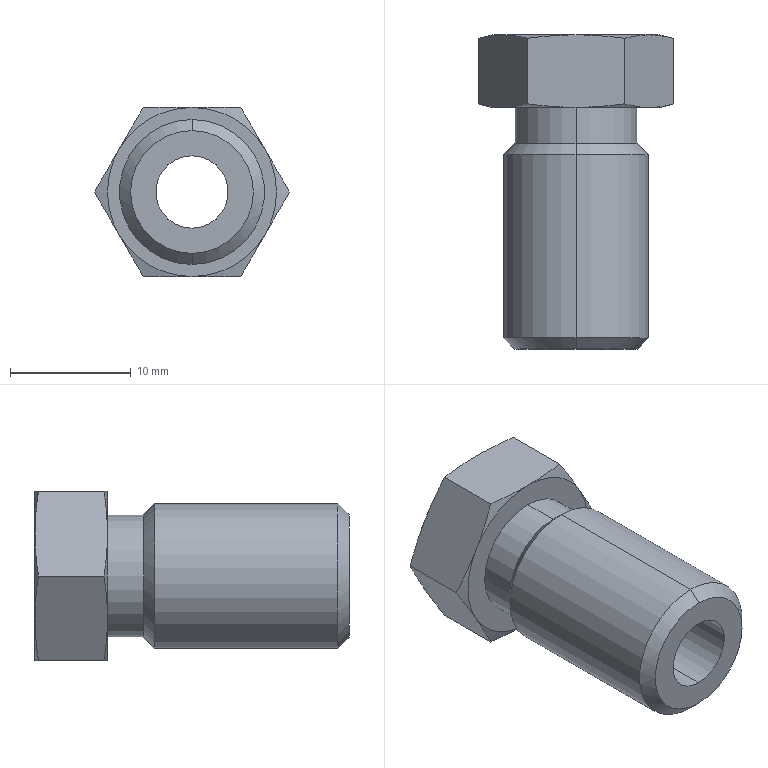Part | SolidWorks | features BaseBody 1 | 1 solid | 32 faces | box 16.166 x 26 x 14 mm | volume 2413 mm3 | cone 16 | plane 10 | cylinder 6 | commonest cylinder face diameters 6 x2 10.1 x2 12 x2
STEP:
#1=CARTESIAN_POINT('',(0.,16.08,-6.));
#2=VERTEX_POINT('',#1);
#3=CARTESIAN_POINT('',(0.,16.08,6.));
#4=VERTEX_POINT('',#3);
#5=CARTESIAN_POINT('',(0.,16.08,0.));
#6=DIRECTION('',(0.,-1.,0.));
#7=DIRECTION('',(0.,0.,-1.));
#8=AXIS2_PLACEMENT_3D('',#5,#6,#7);
#9=CIRCLE('',#8,6.);
#10=EDGE_CURVE('',#2,#4,#9,.T.);
#11=ORIENTED_EDGE('',*,*,#10,.T.);
#12=CARTESIAN_POINT('',(0.,0.92,6.));
#13=VERTEX_POINT('',#12);
#14=CARTESIAN_POINT('',(0.,8.5,6.));
#15=DIRECTION('',(0.,-1.,0.));
#16=VECTOR('',#15,1000.);
#17=LINE('',#14,#16);
#18=EDGE_CURVE('',#4,#13,#17,.T.);
#19=ORIENTED_EDGE('',*,*,#18,.T.);
#20=CARTESIAN_POINT('',(0.,0.92,-6.));
#21=VERTEX_POINT('',#20);
#22=CARTESIAN_POINT('',(0.,0.92,0.));
#23=DIRECTION('',(0.,1.,0.));
#24=DIRECTION('',(0.,0.,-1.));
#25=AXIS2_PLACEMENT_3D('',#22,#23,#24);
#26=CIRCLE('',#25,6.);
#27=EDGE_CURVE('',#13,#21,#26,.T.);
#28=ORIENTED_EDGE('',*,*,#27,.T.);
#29=CARTESIAN_POINT('',(0.,8.5,-6.));
#30=DIRECTION('',(0.,-1.,0.));
#31=VECTOR('',#30,1000.);
#32=LINE('',#29,#31);
#33=EDGE_CURVE('',#2,#21,#32,.T.);
#34=ORIENTED_EDGE('',*,*,#33,.F.);
#35=EDGE_LOOP('',(#11,#19,#28,#34));
#36=FACE_OUTER_BOUND('',#35,.T.);
#37=CARTESIAN_POINT('',(0.,8.5,0.));
#38=DIRECTION('',(0.,-1.,0.));
#39=DIRECTION('',(0.,0.,-1.));
#40=AXIS2_PLACEMENT_3D('',#37,#38,#39);
#41=CYLINDRICAL_SURFACE('',#40,6.);
#42=ADVANCED_FACE('',(#36),#41,.T.);
#43=CARTESIAN_POINT('',(0.,17.,-5.08));
#44=VERTEX_POINT('',#43);
#45=CARTESIAN_POINT('',(0.,17.,5.08));
#46=VERTEX_POINT('',#45);
#47=CARTESIAN_POINT('',(0.,17.,0.));
#48=DIRECTION('',(0.,-1.,0.));
#49=DIRECTION('',(0.,0.,-1.));
#50=AXIS2_PLACEMENT_3D('',#47,#48,#49);
#51=CIRCLE('',#50,5.08);
#52=EDGE_CURVE('',#44,#46,#51,.T.);
#53=ORIENTED_EDGE('',*,*,#52,.T.);
#54=CARTESIAN_POINT('',(0.,16.08,6.));
#55=DIRECTION('',(0.,-0.7071,0.7071));
#56=VECTOR('',#55,1000.);
#57=LINE('',#54,#56);
#58=EDGE_CURVE('',#46,#4,#57,.T.);
#59=ORIENTED_EDGE('',*,*,#58,.T.);
#60=ORIENTED_EDGE('',*,*,#10,.F.);
#61=CARTESIAN_POINT('',(0.,16.08,-6.));
#62=DIRECTION('',(0.,-0.7071,-0.7071));
#63=VECTOR('',#62,1000.);
#64=LINE('',#61,#63);
#65=EDGE_CURVE('',#44,#2,#64,.T.);
#66=ORIENTED_EDGE('',*,*,#65,.F.);
#67=EDGE_LOOP('',(#53,#59,#60,#66));
#68=FACE_OUTER_BOUND('',#67,.T.);
#69=CARTESIAN_POINT('',(0.,16.08,0.));
#70=DIRECTION('',(0.,-1.,0.));
#71=DIRECTION('',(0.,0.,-1.));
#72=AXIS2_PLACEMENT_3D('',#69,#70,#71);
#73=CONICAL_SURFACE('',#72,6.,0.7854);
#74=ADVANCED_FACE('',(#68),#73,.T.);
#75=CARTESIAN_POINT('',(0.,0.,5.08));
#76=VERTEX_POINT('',#75);
#77=CARTESIAN_POINT('',(0.,0.,-5.08));
#78=VERTEX_POINT('',#77);
#79=CARTESIAN_POINT('',(0.,0.,0.));
#80=DIRECTION('',(0.,1.,0.));
#81=DIRECTION('',(0.,0.,1.));
#82=AXIS2_PLACEMENT_3D('',#79,#80,#81);
#83=CIRCLE('',#82,5.08);
#84=EDGE_CURVE('',#76,#78,#83,.T.);
#85=ORIENTED_EDGE('',*,*,#84,.T.);
#86=CARTESIAN_POINT('',(0.,0.92,-6.));
#87=DIRECTION('',(0.,0.7071,-0.7071));
#88=VECTOR('',#87,1000.);
#89=LINE('',#86,#88);
#90=EDGE_CURVE('',#78,#21,#89,.T.);
#91=ORIENTED_EDGE('',*,*,#90,.T.);
#92=ORIENTED_EDGE('',*,*,#27,.F.);
#93=CARTESIAN_POINT('',(0.,0.92,6.));
#94=DIRECTION('',(0.,0.7071,0.7071));
#95=VECTOR('',#94,1000.);
#96=LINE('',#93,#95);
#97=EDGE_CURVE('',#76,#13,#96,.T.);
#98=ORIENTED_EDGE('',*,*,#97,.F.);
#99=EDGE_LOOP('',(#85,#91,#92,#98));
#100=FACE_OUTER_BOUND('',#99,.T.);
#101=CARTESIAN_POINT('',(0.,0.92,0.));
#102=DIRECTION('',(0.,1.,0.));
#103=DIRECTION('',(0.,0.,1.));
#104=AXIS2_PLACEMENT_3D('',#101,#102,#103);
#105=CONICAL_SURFACE('',#104,6.,0.7854);
#106=ADVANCED_FACE('',(#100),#105,.T.);
#107=CARTESIAN_POINT('',(0.,20.,-5.05));
#108=VERTEX_POINT('',#107);
#109=CARTESIAN_POINT('',(0.,20.,5.05));
#110=VERTEX_POINT('',#109);
#111=CARTESIAN_POINT('',(0.,20.,0.));
#112=DIRECTION('',(0.,-1.,0.));
#113=DIRECTION('',(0.,0.,-1.));
#114=AXIS2_PLACEMENT_3D('',#111,#112,#113);
#115=CIRCLE('',#114,5.05);
#116=EDGE_CURVE('',#108,#110,#115,.T.);
#117=ORIENTED_EDGE('',*,*,#116,.T.);
#118=CARTESIAN_POINT('',(0.,17.,5.05));
#119=VERTEX_POINT('',#118);
#120=CARTESIAN_POINT('',(0.,18.5,5.05));
#121=DIRECTION('',(0.,-1.,0.));
#122=VECTOR('',#121,1000.);
#123=LINE('',#120,#122);
#124=EDGE_CURVE('',#110,#119,#123,.T.);
#125=ORIENTED_EDGE('',*,*,#124,.T.);
#126=CARTESIAN_POINT('',(0.,17.,-5.05));
#127=VERTEX_POINT('',#126);
#128=CARTESIAN_POINT('',(0.,17.,0.));
#129=DIRECTION('',(0.,-1.,0.));
#130=DIRECTION('',(0.,0.,-1.));
#131=AXIS2_PLACEMENT_3D('',#128,#129,#130);
#132=CIRCLE('',#131,5.05);
#133=EDGE_CURVE('',#127,#119,#132,.T.);
#134=ORIENTED_EDGE('',*,*,#133,.F.);
#135=CARTESIAN_POINT('',(0.,18.5,-5.05));
#136=DIRECTION('',(0.,-1.,0.));
#137=VECTOR('',#136,1000.);
#138=LINE('',#135,#137);
#139=EDGE_CURVE('',#108,#127,#138,.T.);
#140=ORIENTED_EDGE('',*,*,#139,.F.);
#141=EDGE_LOOP('',(#117,#125,#134,#140));
#142=FACE_OUTER_BOUND('',#141,.T.);
#143=CARTESIAN_POINT('',(0.,18.5,0.));
#144=DIRECTION('',(0.,-1.,0.));
#145=DIRECTION('',(0.,0.,-1.));
#146=AXIS2_PLACEMENT_3D('',#143,#144,#145);
#147=CYLINDRICAL_SURFACE('',#146,5.05);
#148=ADVANCED_FACE('',(#142),#147,.T.);
#149=CARTESIAN_POINT('',(0.,26.,3.));
#150=VERTEX_POINT('',#149);
#151=CARTESIAN_POINT('',(0.,26.,-3.));
#152=VERTEX_POINT('',#151);
#153=CARTESIAN_POINT('',(0.,26.,0.));
#154=DIRECTION('',(0.,-1.,0.));
#155=DIRECTION('',(0.,0.,-1.));
#156=AXIS2_PLACEMENT_3D('',#153,#154,#155);
#157=CIRCLE('',#156,3.);
#158=EDGE_CURVE('',#150,#152,#157,.T.);
#159=ORIENTED_EDGE('',*,*,#158,.F.);
#160=CARTESIAN_POINT('',(0.,0.,3.));
#161=VERTEX_POINT('',#160);
#162=CARTESIAN_POINT('',(0.,13.,3.));
#163=DIRECTION('',(0.,-1.,0.));
#164=VECTOR('',#163,1000.);
#165=LINE('',#162,#164);
#166=EDGE_CURVE('',#150,#161,#165,.T.);
#167=ORIENTED_EDGE('',*,*,#166,.T.);
#168=CARTESIAN_POINT('',(0.,0.,-3.));
#169=VERTEX_POINT('',#168);
#170=CARTESIAN_POINT('',(0.,0.,0.));
#171=DIRECTION('',(0.,1.,0.));
#172=DIRECTION('',(0.,0.,-1.));
#173=AXIS2_PLACEMENT_3D('',#170,#171,#172);
#174=CIRCLE('',#173,3.);
#175=EDGE_CURVE('',#169,#161,#174,.T.);
#176=ORIENTED_EDGE('',*,*,#175,.F.);
#177=CARTESIAN_POINT('',(0.,13.,-3.));
#178=DIRECTION('',(0.,-1.,0.));
#179=VECTOR('',#178,1000.);
#180=LINE('',#177,#179);
#181=EDGE_CURVE('',#152,#169,#180,.T.);
#182=ORIENTED_EDGE('',*,*,#181,.F.);
#183=EDGE_LOOP('',(#159,#167,#176,#182));
#184=FACE_OUTER_BOUND('',#183,.T.);
#185=CARTESIAN_POINT('',(0.,13.,0.));
#186=DIRECTION('',(0.,-1.,0.));
#187=DIRECTION('',(0.,0.,-1.));
#188=AXIS2_PLACEMENT_3D('',#185,#186,#187);
#189=CYLINDRICAL_SURFACE('',#188,3.);
#190=ADVANCED_FACE('',(#184),#189,.F.);
#191=ORIENTED_EDGE('',*,*,#18,.F.);
#192=CARTESIAN_POINT('',(0.,16.08,0.));
#193=DIRECTION('',(0.,-1.,0.));
#194=DIRECTION('',(0.,0.,-1.));
#195=AXIS2_PLACEMENT_3D('',#192,#193,#194);
#196=CIRCLE('',#195,6.);
#197=EDGE_CURVE('',#4,#2,#196,.T.);
#198=ORIENTED_EDGE('',*,*,#197,.T.);
#199=ORIENTED_EDGE('',*,*,#33,.T.);
#200=CARTESIAN_POINT('',(0.,0.92,0.));
#201=DIRECTION('',(0.,1.,0.));
#202=DIRECTION('',(0.,0.,-1.));
#203=AXIS2_PLACEMENT_3D('',#200,#201,#202);
#204=CIRCLE('',#203,6.);
#205=EDGE_CURVE('',#21,#13,#204,.T.);
#206=ORIENTED_EDGE('',*,*,#205,.T.);
#207=EDGE_LOOP('',(#191,#198,#199,#206));
#208=FACE_OUTER_BOUND('',#207,.T.);
#209=CARTESIAN_POINT('',(0.,8.5,0.));
#210=DIRECTION('',(0.,-1.,0.));
#211=DIRECTION('',(0.,0.,-1.));
#212=AXIS2_PLACEMENT_3D('',#209,#210,#211);
#213=CYLINDRICAL_SURFACE('',#212,6.);
#214=ADVANCED_FACE('',(#208),#213,.T.);
#215=ORIENTED_EDGE('',*,*,#58,.F.);
#216=CARTESIAN_POINT('',(0.,17.,0.));
#217=DIRECTION('',(0.,-1.,0.));
#218=DIRECTION('',(0.,0.,-1.));
#219=AXIS2_PLACEMENT_3D('',#216,#217,#218);
#220=CIRCLE('',#219,5.08);
#221=EDGE_CURVE('',#46,#44,#220,.T.);
#222=ORIENTED_EDGE('',*,*,#221,.T.);
#223=ORIENTED_EDGE('',*,*,#65,.T.);
#224=ORIENTED_EDGE('',*,*,#197,.F.);
#225=EDGE_LOOP('',(#215,#222,#223,#224));
#226=FACE_OUTER_BOUND('',#225,.T.);
#227=CARTESIAN_POINT('',(0.,16.08,0.));
#228=DIRECTION('',(0.,-1.,0.));
#229=DIRECTION('',(0.,0.,-1.));
#230=AXIS2_PLACEMENT_3D('',#227,#228,#229);
#231=CONICAL_SURFACE('',#230,6.,0.7854);
#232=ADVANCED_FACE('',(#226),#231,.T.);
#233=ORIENTED_EDGE('',*,*,#90,.F.);
#234=CARTESIAN_POINT('',(0.,0.,0.));
#235=DIRECTION('',(0.,1.,0.));
#236=DIRECTION('',(0.,0.,1.));
#237=AXIS2_PLACEMENT_3D('',#234,#235,#236);
#238=CIRCLE('',#237,5.08);
#239=EDGE_CURVE('',#78,#76,#238,.T.);
#240=ORIENTED_EDGE('',*,*,#239,.T.);
#241=ORIENTED_EDGE('',*,*,#97,.T.);
#242=ORIENTED_EDGE('',*,*,#205,.F.);
#243=EDGE_LOOP('',(#233,#240,#241,#242));
#244=FACE_OUTER_BOUND('',#243,.T.);
#245=CARTESIAN_POINT('',(0.,0.92,0.));
#246=DIRECTION('',(0.,1.,0.));
#247=DIRECTION('',(0.,0.,1.));
#248=AXIS2_PLACEMENT_3D('',#245,#246,#247);
#249=CONICAL_SURFACE('',#248,6.,0.7854);
#250=ADVANCED_FACE('',(#244),#249,.T.);
#251=ORIENTED_EDGE('',*,*,#52,.F.);
#252=ORIENTED_EDGE('',*,*,#221,.F.);
#253=EDGE_LOOP('',(#251,#252));
#254=FACE_OUTER_BOUND('',#253,.T.);
#255=ORIENTED_EDGE('',*,*,#133,.T.);
#256=CARTESIAN_POINT('',(0.,17.,0.));
#257=DIRECTION('',(0.,-1.,0.));
#258=DIRECTION('',(0.,0.,-1.));
#259=AXIS2_PLACEMENT_3D('',#256,#257,#258);
#260=CIRCLE('',#259,5.05);
#261=EDGE_CURVE('',#119,#127,#260,.T.);
#262=ORIENTED_EDGE('',*,*,#261,.T.);
#263=EDGE_LOOP('',(#255,#262));
#264=FACE_BOUND('',#263,.T.);
#265=CARTESIAN_POINT('',(5.065,17.,0.));
#266=DIRECTION('',(0.,1.,0.));
#267=DIRECTION('',(0.,0.,1.));
#268=AXIS2_PLACEMENT_3D('',#265,#266,#267);
#269=PLANE('',#268);
#270=ADVANCED_FACE('',(#254,#264),#269,.T.);
#271=ORIENTED_EDGE('',*,*,#84,.F.);
#272=ORIENTED_EDGE('',*,*,#239,.F.);
#273=EDGE_LOOP('',(#271,#272));
#274=FACE_OUTER_BOUND('',#273,.T.);
#275=ORIENTED_EDGE('',*,*,#175,.T.);
#276=CARTESIAN_POINT('',(0.,0.,0.));
#277=DIRECTION('',(0.,1.,0.));
#278=DIRECTION('',(0.,0.,-1.));
#279=AXIS2_PLACEMENT_3D('',#276,#277,#278);
#280=CIRCLE('',#279,3.);
#281=EDGE_CURVE('',#161,#169,#280,.T.);
#282=ORIENTED_EDGE('',*,*,#281,.T.);
#283=EDGE_LOOP('',(#275,#282));
#284=FACE_BOUND('',#283,.T.);
#285=CARTESIAN_POINT('',(2.54,0.,0.));
#286=DIRECTION('',(0.,-1.,0.));
#287=DIRECTION('',(0.,0.,-1.));
#288=AXIS2_PLACEMENT_3D('',#285,#286,#287);
#289=PLANE('',#288);
#290=ADVANCED_FACE('',(#274,#284),#289,.T.);
#291=ORIENTED_EDGE('',*,*,#124,.F.);
#292=CARTESIAN_POINT('',(0.,20.,0.));
#293=DIRECTION('',(0.,-1.,0.));
#294=DIRECTION('',(0.,0.,-1.));
#295=AXIS2_PLACEMENT_3D('',#292,#293,#294);
#296=CIRCLE('',#295,5.05);
#297=EDGE_CURVE('',#110,#108,#296,.T.);
#298=ORIENTED_EDGE('',*,*,#297,.T.);
#299=ORIENTED_EDGE('',*,*,#139,.T.);
#300=ORIENTED_EDGE('',*,*,#261,.F.);
#301=EDGE_LOOP('',(#291,#298,#299,#300));
#302=FACE_OUTER_BOUND('',#301,.T.);
#303=CARTESIAN_POINT('',(0.,18.5,0.));
#304=DIRECTION('',(0.,-1.,0.));
#305=DIRECTION('',(0.,0.,-1.));
#306=AXIS2_PLACEMENT_3D('',#303,#304,#305);
#307=CYLINDRICAL_SURFACE('',#306,5.05);
#308=ADVANCED_FACE('',(#302),#307,.T.);
#309=ORIENTED_EDGE('',*,*,#166,.F.);
#310=CARTESIAN_POINT('',(0.,26.,0.));
#311=DIRECTION('',(0.,-1.,0.));
#312=DIRECTION('',(0.,0.,-1.));
#313=AXIS2_PLACEMENT_3D('',#310,#311,#312);
#314=CIRCLE('',#313,3.);
#315=EDGE_CURVE('',#152,#150,#314,.T.);
#316=ORIENTED_EDGE('',*,*,#315,.F.);
#317=ORIENTED_EDGE('',*,*,#181,.T.);
#318=ORIENTED_EDGE('',*,*,#281,.F.);
#319=EDGE_LOOP('',(#309,#316,#317,#318));
#320=FACE_OUTER_BOUND('',#319,.T.);
#321=CARTESIAN_POINT('',(0.,13.,0.));
#322=DIRECTION('',(0.,-1.,0.));
#323=DIRECTION('',(0.,0.,-1.));
#324=AXIS2_PLACEMENT_3D('',#321,#322,#323);
#325=CYLINDRICAL_SURFACE('',#324,3.);
#326=ADVANCED_FACE('',(#320),#325,.F.);
#327=ORIENTED_EDGE('',*,*,#116,.F.);
#328=ORIENTED_EDGE('',*,*,#297,.F.);
#329=EDGE_LOOP('',(#327,#328));
#330=FACE_BOUND('',#329,.T.);
#331=CARTESIAN_POINT('',(0.,20.,-7.));
#332=VERTEX_POINT('',#331);
#333=CARTESIAN_POINT('',(6.062,20.,-3.5));
#334=VERTEX_POINT('',#333);
#335=CARTESIAN_POINT('',(0.,20.,0.));
#336=DIRECTION('',(0.,-1.,0.));
#337=DIRECTION('',(0.,0.,1.));
#338=AXIS2_PLACEMENT_3D('',#335,#336,#337);
#339=CIRCLE('',#338,7.);
#340=EDGE_CURVE('',#332,#334,#339,.T.);
#341=ORIENTED_EDGE('',*,*,#340,.T.);
#342=CARTESIAN_POINT('',(6.062,20.,3.5));
#343=VERTEX_POINT('',#342);
#344=CARTESIAN_POINT('',(0.,20.,0.));
#345=DIRECTION('',(0.,-1.,0.));
#346=DIRECTION('',(0.,0.,1.));
#347=AXIS2_PLACEMENT_3D('',#344,#345,#346);
#348=CIRCLE('',#347,7.);
#349=EDGE_CURVE('',#334,#343,#348,.T.);
#350=ORIENTED_EDGE('',*,*,#349,.T.);
#351=CARTESIAN_POINT('',(0.,20.,7.));
#352=VERTEX_POINT('',#351);
#353=CARTESIAN_POINT('',(0.,20.,0.));
#354=DIRECTION('',(0.,-1.,0.));
#355=DIRECTION('',(0.,0.,1.));
#356=AXIS2_PLACEMENT_3D('',#353,#354,#355);
#357=CIRCLE('',#356,7.);
#358=EDGE_CURVE('',#343,#352,#357,.T.);
#359=ORIENTED_EDGE('',*,*,#358,.T.);
#360=CARTESIAN_POINT('',(-6.062,20.,3.5));
#361=VERTEX_POINT('',#360);
#362=CARTESIAN_POINT('',(0.,20.,0.));
#363=DIRECTION('',(0.,-1.,0.));
#364=DIRECTION('',(0.,0.,1.));
#365=AXIS2_PLACEMENT_3D('',#362,#363,#364);
#366=CIRCLE('',#365,7.);
#367=EDGE_CURVE('',#352,#361,#366,.T.);
#368=ORIENTED_EDGE('',*,*,#367,.T.);
#369=CARTESIAN_POINT('',(-6.062,20.,-3.5));
#370=VERTEX_POINT('',#369);
#371=CARTESIAN_POINT('',(0.,20.,0.));
#372=DIRECTION('',(0.,-1.,0.));
#373=DIRECTION('',(0.,0.,1.));
#374=AXIS2_PLACEMENT_3D('',#371,#372,#373);
#375=CIRCLE('',#374,7.);
#376=EDGE_CURVE('',#361,#370,#375,.T.);
#377=ORIENTED_EDGE('',*,*,#376,.T.);
#378=CARTESIAN_POINT('',(0.,20.,0.));
#379=DIRECTION('',(0.,-1.,0.));
#380=DIRECTION('',(0.,0.,1.));
#381=AXIS2_PLACEMENT_3D('',#378,#379,#380);
#382=CIRCLE('',#381,7.);
#383=EDGE_CURVE('',#370,#332,#382,.T.);
#384=ORIENTED_EDGE('',*,*,#383,.T.);
#385=EDGE_LOOP('',(#341,#350,#359,#368,#377,#384));
#386=FACE_OUTER_BOUND('',#385,.T.);
#387=CARTESIAN_POINT('',(6.025,20.,0.));
#388=DIRECTION('',(0.,-1.,0.));
#389=DIRECTION('',(0.,0.,-1.));
#390=AXIS2_PLACEMENT_3D('',#387,#388,#389);
#391=PLANE('',#390);
#392=ADVANCED_FACE('',(#330,#386),#391,.T.);
#393=CARTESIAN_POINT('',(-6.062,26.,3.5));
#394=VERTEX_POINT('',#393);
#395=CARTESIAN_POINT('',(0.,26.,7.));
#396=VERTEX_POINT('',#395);
#397=CARTESIAN_POINT('',(0.,26.,0.));
#398=DIRECTION('',(0.,1.,0.));
#399=DIRECTION('',(0.,0.,-1.));
#400=AXIS2_PLACEMENT_3D('',#397,#398,#399);
#401=CIRCLE('',#400,7.);
#402=EDGE_CURVE('',#394,#396,#401,.T.);
#403=ORIENTED_EDGE('',*,*,#402,.T.);
#404=CARTESIAN_POINT('',(6.062,26.,3.5));
#405=VERTEX_POINT('',#404);
#406=CARTESIAN_POINT('',(0.,26.,0.));
#407=DIRECTION('',(0.,1.,0.));
#408=DIRECTION('',(0.,0.,-1.));
#409=AXIS2_PLACEMENT_3D('',#406,#407,#408);
#410=CIRCLE('',#409,7.);
#411=EDGE_CURVE('',#396,#405,#410,.T.);
#412=ORIENTED_EDGE('',*,*,#411,.T.);
#413=CARTESIAN_POINT('',(6.062,26.,-3.5));
#414=VERTEX_POINT('',#413);
#415=CARTESIAN_POINT('',(0.,26.,0.));
#416=DIRECTION('',(0.,1.,0.));
#417=DIRECTION('',(0.,0.,-1.));
#418=AXIS2_PLACEMENT_3D('',#415,#416,#417);
#419=CIRCLE('',#418,7.);
#420=EDGE_CURVE('',#405,#414,#419,.T.);
#421=ORIENTED_EDGE('',*,*,#420,.T.);
#422=CARTESIAN_POINT('',(0.,26.,-7.));
#423=VERTEX_POINT('',#422);
#424=CARTESIAN_POINT('',(0.,26.,0.));
#425=DIRECTION('',(0.,1.,0.));
#426=DIRECTION('',(0.,0.,-1.));
#427=AXIS2_PLACEMENT_3D('',#424,#425,#426);
#428=CIRCLE('',#427,7.);
#429=EDGE_CURVE('',#414,#423,#428,.T.);
#430=ORIENTED_EDGE('',*,*,#429,.T.);
#431=CARTESIAN_POINT('',(-6.062,26.,-3.5));
#432=VERTEX_POINT('',#431);
#433=CARTESIAN_POINT('',(0.,26.,0.));
#434=DIRECTION('',(0.,1.,0.));
#435=DIRECTION('',(0.,0.,-1.));
#436=AXIS2_PLACEMENT_3D('',#433,#434,#435);
#437=CIRCLE('',#436,7.);
#438=EDGE_CURVE('',#423,#432,#437,.T.);
#439=ORIENTED_EDGE('',*,*,#438,.T.);
#440=CARTESIAN_POINT('',(0.,26.,0.));
#441=DIRECTION('',(0.,1.,0.));
#442=DIRECTION('',(0.,0.,-1.));
#443=AXIS2_PLACEMENT_3D('',#440,#441,#442);
#444=CIRCLE('',#443,7.);
#445=EDGE_CURVE('',#432,#394,#444,.T.);
#446=ORIENTED_EDGE('',*,*,#445,.T.);
#447=EDGE_LOOP('',(#403,#412,#421,#430,#439,#446));
#448=FACE_OUTER_BOUND('',#447,.T.);
#449=ORIENTED_EDGE('',*,*,#315,.T.);
#450=ORIENTED_EDGE('',*,*,#158,.T.);
#451=EDGE_LOOP('',(#449,#450));
#452=FACE_BOUND('',#451,.T.);
#453=CARTESIAN_POINT('',(3.5,26.,0.));
#454=DIRECTION('',(0.,1.,0.));
#455=DIRECTION('',(0.,0.,1.));
#456=AXIS2_PLACEMENT_3D('',#453,#454,#455);
#457=PLANE('',#456);
#458=ADVANCED_FACE('',(#448,#452),#457,.T.);
#459=ORIENTED_EDGE('',*,*,#349,.F.);
#460=CARTESIAN_POINT('',(8.083,20.29,0.));
#461=VERTEX_POINT('',#460);
#462=CARTESIAN_POINT('',(6.062,20.,-3.5));
#463=CARTESIAN_POINT('',(6.739,20.,-2.327));
#464=CARTESIAN_POINT('',(7.412,20.11,-1.162));
#465=CARTESIAN_POINT('',(8.083,20.29,0.));
#466=B_SPLINE_CURVE_WITH_KNOTS('',3,(#462,#463,#464,#465),.UNSPECIFIED.,.F.,.F.,(4,4),(0.,0.004052),.UNSPECIFIED.);
#467=EDGE_CURVE('',#334,#461,#466,.T.);
#468=ORIENTED_EDGE('',*,*,#467,.T.);
#469=CARTESIAN_POINT('',(8.083,20.29,0.));
#470=CARTESIAN_POINT('',(7.412,20.11,1.162));
#471=CARTESIAN_POINT('',(6.739,20.,2.327));
#472=CARTESIAN_POINT('',(6.062,20.,3.5));
#473=B_SPLINE_CURVE_WITH_KNOTS('',3,(#469,#470,#471,#472),.UNSPECIFIED.,.F.,.F.,(4,4),(0.,0.004052),.UNSPECIFIED.);
#474=EDGE_CURVE('',#461,#343,#473,.T.);
#475=ORIENTED_EDGE('',*,*,#474,.T.);
#476=EDGE_LOOP('',(#459,#468,#475));
#477=FACE_OUTER_BOUND('',#476,.T.);
#478=CARTESIAN_POINT('',(0.,20.292,0.));
#479=DIRECTION('',(0.,1.,0.));
#480=DIRECTION('',(0.,0.,1.));
#481=AXIS2_PLACEMENT_3D('',#478,#479,#480);
#482=CONICAL_SURFACE('',#481,8.089,1.309);
#483=ADVANCED_FACE('',(#477),#482,.T.);
#484=ORIENTED_EDGE('',*,*,#340,.F.);
#485=CARTESIAN_POINT('',(4.041,20.29,-7.));
#486=VERTEX_POINT('',#485);
#487=CARTESIAN_POINT('',(0.,20.,-7.));
#488=CARTESIAN_POINT('',(1.354,20.,-7.));
#489=CARTESIAN_POINT('',(2.7,20.11,-7.));
#490=CARTESIAN_POINT('',(4.041,20.29,-7.));
#491=B_SPLINE_CURVE_WITH_KNOTS('',3,(#487,#488,#489,#490),.UNSPECIFIED.,.F.,.F.,(4,4),(0.,0.004052),.UNSPECIFIED.);
#492=EDGE_CURVE('',#332,#486,#491,.T.);
#493=ORIENTED_EDGE('',*,*,#492,.T.);
#494=CARTESIAN_POINT('',(4.041,20.29,-7.));
#495=CARTESIAN_POINT('',(4.712,20.11,-5.838));
#496=CARTESIAN_POINT('',(5.385,20.,-4.673));
#497=CARTESIAN_POINT('',(6.062,20.,-3.5));
#498=B_SPLINE_CURVE_WITH_KNOTS('',3,(#494,#495,#496,#497),.UNSPECIFIED.,.F.,.F.,(4,4),(0.,0.004052),.UNSPECIFIED.);
#499=EDGE_CURVE('',#486,#334,#498,.T.);
#500=ORIENTED_EDGE('',*,*,#499,.T.);
#501=EDGE_LOOP('',(#484,#493,#500));
#502=FACE_OUTER_BOUND('',#501,.T.);
#503=CARTESIAN_POINT('',(0.,20.292,0.));
#504=DIRECTION('',(0.,1.,0.));
#505=DIRECTION('',(0.,0.,1.));
#506=AXIS2_PLACEMENT_3D('',#503,#504,#505);
#507=CONICAL_SURFACE('',#506,8.089,1.309);
#508=ADVANCED_FACE('',(#502),#507,.T.);
#509=CARTESIAN_POINT('',(-4.041,20.29,-7.));
#510=VERTEX_POINT('',#509);
#511=CARTESIAN_POINT('',(-4.041,20.29,-7.));
#512=CARTESIAN_POINT('',(-2.7,20.11,-7.));
#513=CARTESIAN_POINT('',(-1.354,20.,-7.));
#514=CARTESIAN_POINT('',(0.,20.,-7.));
#515=B_SPLINE_CURVE_WITH_KNOTS('',3,(#511,#512,#513,#514),.UNSPECIFIED.,.F.,.F.,(4,4),(0.,0.004052),.UNSPECIFIED.);
#516=EDGE_CURVE('',#510,#332,#515,.T.);
#517=ORIENTED_EDGE('',*,*,#516,.T.);
#518=ORIENTED_EDGE('',*,*,#383,.F.);
#519=CARTESIAN_POINT('',(-6.062,20.,-3.5));
#520=CARTESIAN_POINT('',(-5.385,20.,-4.673));
#521=CARTESIAN_POINT('',(-4.712,20.11,-5.838));
#522=CARTESIAN_POINT('',(-4.041,20.29,-7.));
#523=B_SPLINE_CURVE_WITH_KNOTS('',3,(#519,#520,#521,#522),.UNSPECIFIED.,.F.,.F.,(4,4),(0.,0.004052),.UNSPECIFIED.);
#524=EDGE_CURVE('',#370,#510,#523,.T.);
#525=ORIENTED_EDGE('',*,*,#524,.T.);
#526=EDGE_LOOP('',(#517,#518,#525));
#527=FACE_OUTER_BOUND('',#526,.T.);
#528=CARTESIAN_POINT('',(0.,20.292,0.));
#529=DIRECTION('',(0.,1.,0.));
#530=DIRECTION('',(0.,0.,1.));
#531=AXIS2_PLACEMENT_3D('',#528,#529,#530);
#532=CONICAL_SURFACE('',#531,8.089,1.309);
#533=ADVANCED_FACE('',(#527),#532,.T.);
#534=CARTESIAN_POINT('',(-8.083,20.29,0.));
#535=VERTEX_POINT('',#534);
#536=CARTESIAN_POINT('',(-8.083,20.29,0.));
#537=CARTESIAN_POINT('',(-7.412,20.11,-1.162));
#538=CARTESIAN_POINT('',(-6.739,20.,-2.327));
#539=CARTESIAN_POINT('',(-6.062,20.,-3.5));
#540=B_SPLINE_CURVE_WITH_KNOTS('',3,(#536,#537,#538,#539),.UNSPECIFIED.,.F.,.F.,(4,4),(0.,0.004052),.UNSPECIFIED.);
#541=EDGE_CURVE('',#535,#370,#540,.T.);
#542=ORIENTED_EDGE('',*,*,#541,.T.);
#543=ORIENTED_EDGE('',*,*,#376,.F.);
#544=CARTESIAN_POINT('',(-6.062,20.,3.5));
#545=CARTESIAN_POINT('',(-6.739,20.,2.327));
#546=CARTESIAN_POINT('',(-7.412,20.11,1.162));
#547=CARTESIAN_POINT('',(-8.083,20.29,0.));
#548=B_SPLINE_CURVE_WITH_KNOTS('',3,(#544,#545,#546,#547),.UNSPECIFIED.,.F.,.F.,(4,4),(0.,0.004052),.UNSPECIFIED.);
#549=EDGE_CURVE('',#361,#535,#548,.T.);
#550=ORIENTED_EDGE('',*,*,#549,.T.);
#551=EDGE_LOOP('',(#542,#543,#550));
#552=FACE_OUTER_BOUND('',#551,.T.);
#553=CARTESIAN_POINT('',(0.,20.292,0.));
#554=DIRECTION('',(0.,1.,0.));
#555=DIRECTION('',(0.,0.,1.));
#556=AXIS2_PLACEMENT_3D('',#553,#554,#555);
#557=CONICAL_SURFACE('',#556,8.089,1.309);
#558=ADVANCED_FACE('',(#552),#557,.T.);
#559=CARTESIAN_POINT('',(-4.041,20.29,7.));
#560=VERTEX_POINT('',#559);
#561=CARTESIAN_POINT('',(-4.041,20.29,7.));
#562=CARTESIAN_POINT('',(-4.712,20.11,5.838));
#563=CARTESIAN_POINT('',(-5.385,20.,4.673));
#564=CARTESIAN_POINT('',(-6.062,20.,3.5));
#565=B_SPLINE_CURVE_WITH_KNOTS('',3,(#561,#562,#563,#564),.UNSPECIFIED.,.F.,.F.,(4,4),(0.,0.004052),.UNSPECIFIED.);
#566=EDGE_CURVE('',#560,#361,#565,.T.);
#567=ORIENTED_EDGE('',*,*,#566,.T.);
#568=ORIENTED_EDGE('',*,*,#367,.F.);
#569=CARTESIAN_POINT('',(0.,20.,7.));
#570=CARTESIAN_POINT('',(-1.354,20.,7.));
#571=CARTESIAN_POINT('',(-2.7,20.11,7.));
#572=CARTESIAN_POINT('',(-4.041,20.29,7.));
#573=B_SPLINE_CURVE_WITH_KNOTS('',3,(#569,#570,#571,#572),.UNSPECIFIED.,.F.,.F.,(4,4),(0.,0.004052),.UNSPECIFIED.);
#574=EDGE_CURVE('',#352,#560,#573,.T.);
#575=ORIENTED_EDGE('',*,*,#574,.T.);
#576=EDGE_LOOP('',(#567,#568,#575));
#577=FACE_OUTER_BOUND('',#576,.T.);
#578=CARTESIAN_POINT('',(0.,20.292,0.));
#579=DIRECTION('',(0.,1.,0.));
#580=DIRECTION('',(0.,0.,1.));
#581=AXIS2_PLACEMENT_3D('',#578,#579,#580);
#582=CONICAL_SURFACE('',#581,8.089,1.309);
#583=ADVANCED_FACE('',(#577),#582,.T.);
#584=ORIENTED_EDGE('',*,*,#358,.F.);
#585=CARTESIAN_POINT('',(4.041,20.29,7.));
#586=VERTEX_POINT('',#585);
#587=CARTESIAN_POINT('',(6.062,20.,3.5));
#588=CARTESIAN_POINT('',(5.385,20.,4.673));
#589=CARTESIAN_POINT('',(4.712,20.11,5.838));
#590=CARTESIAN_POINT('',(4.041,20.29,7.));
#591=B_SPLINE_CURVE_WITH_KNOTS('',3,(#587,#588,#589,#590),.UNSPECIFIED.,.F.,.F.,(4,4),(0.,0.004052),.UNSPECIFIED.);
#592=EDGE_CURVE('',#343,#586,#591,.T.);
#593=ORIENTED_EDGE('',*,*,#592,.T.);
#594=CARTESIAN_POINT('',(4.041,20.29,7.));
#595=CARTESIAN_POINT('',(2.7,20.11,7.));
#596=CARTESIAN_POINT('',(1.354,20.,7.));
#597=CARTESIAN_POINT('',(0.,20.,7.));
#598=B_SPLINE_CURVE_WITH_KNOTS('',3,(#594,#595,#596,#597),.UNSPECIFIED.,.F.,.F.,(4,4),(0.,0.004052),.UNSPECIFIED.);
#599=EDGE_CURVE('',#586,#352,#598,.T.);
#600=ORIENTED_EDGE('',*,*,#599,.T.);
#601=EDGE_LOOP('',(#584,#593,#600));
#602=FACE_OUTER_BOUND('',#601,.T.);
#603=CARTESIAN_POINT('',(0.,20.292,0.));
#604=DIRECTION('',(0.,1.,0.));
#605=DIRECTION('',(0.,0.,1.));
#606=AXIS2_PLACEMENT_3D('',#603,#604,#605);
#607=CONICAL_SURFACE('',#606,8.089,1.309);
#608=ADVANCED_FACE('',(#602),#607,.T.);
#609=ORIENTED_EDGE('',*,*,#411,.F.);
#610=CARTESIAN_POINT('',(4.041,25.71,7.));
#611=VERTEX_POINT('',#610);
#612=CARTESIAN_POINT('',(0.,26.,7.));
#613=CARTESIAN_POINT('',(1.354,26.,7.));
#614=CARTESIAN_POINT('',(2.7,25.89,7.));
#615=CARTESIAN_POINT('',(4.041,25.71,7.));
#616=B_SPLINE_CURVE_WITH_KNOTS('',3,(#612,#613,#614,#615),.UNSPECIFIED.,.F.,.F.,(4,4),(0.,0.004052),.UNSPECIFIED.);
#617=EDGE_CURVE('',#396,#611,#616,.T.);
#618=ORIENTED_EDGE('',*,*,#617,.T.);
#619=CARTESIAN_POINT('',(4.041,25.71,7.));
#620=CARTESIAN_POINT('',(4.712,25.89,5.838));
#621=CARTESIAN_POINT('',(5.385,26.,4.673));
#622=CARTESIAN_POINT('',(6.062,26.,3.5));
#623=B_SPLINE_CURVE_WITH_KNOTS('',3,(#619,#620,#621,#622),.UNSPECIFIED.,.F.,.F.,(4,4),(0.,0.004052),.UNSPECIFIED.);
#624=EDGE_CURVE('',#611,#405,#623,.T.);
#625=ORIENTED_EDGE('',*,*,#624,.T.);
#626=EDGE_LOOP('',(#609,#618,#625));
#627=FACE_OUTER_BOUND('',#626,.T.);
#628=CARTESIAN_POINT('',(0.,25.708,0.));
#629=DIRECTION('',(0.,-1.,0.));
#630=DIRECTION('',(0.,0.,-1.));
#631=AXIS2_PLACEMENT_3D('',#628,#629,#630);
#632=CONICAL_SURFACE('',#631,8.089,1.309);
#633=ADVANCED_FACE('',(#627),#632,.T.);
#634=ORIENTED_EDGE('',*,*,#402,.F.);
#635=CARTESIAN_POINT('',(-4.041,25.71,7.));
#636=VERTEX_POINT('',#635);
#637=CARTESIAN_POINT('',(-6.062,26.,3.5));
#638=CARTESIAN_POINT('',(-5.385,26.,4.673));
#639=CARTESIAN_POINT('',(-4.712,25.89,5.838));
#640=CARTESIAN_POINT('',(-4.041,25.71,7.));
#641=B_SPLINE_CURVE_WITH_KNOTS('',3,(#637,#638,#639,#640),.UNSPECIFIED.,.F.,.F.,(4,4),(0.,0.004052),.UNSPECIFIED.);
#642=EDGE_CURVE('',#394,#636,#641,.T.);
#643=ORIENTED_EDGE('',*,*,#642,.T.);
#644=CARTESIAN_POINT('',(-4.041,25.71,7.));
#645=CARTESIAN_POINT('',(-2.7,25.89,7.));
#646=CARTESIAN_POINT('',(-1.354,26.,7.));
#647=CARTESIAN_POINT('',(0.,26.,7.));
#648=B_SPLINE_CURVE_WITH_KNOTS('',3,(#644,#645,#646,#647),.UNSPECIFIED.,.F.,.F.,(4,4),(0.,0.004052),.UNSPECIFIED.);
#649=EDGE_CURVE('',#636,#396,#648,.T.);
#650=ORIENTED_EDGE('',*,*,#649,.T.);
#651=EDGE_LOOP('',(#634,#643,#650));
#652=FACE_OUTER_BOUND('',#651,.T.);
#653=CARTESIAN_POINT('',(0.,25.708,0.));
#654=DIRECTION('',(0.,-1.,0.));
#655=DIRECTION('',(0.,0.,-1.));
#656=AXIS2_PLACEMENT_3D('',#653,#654,#655);
#657=CONICAL_SURFACE('',#656,8.089,1.309);
#658=ADVANCED_FACE('',(#652),#657,.T.);
#659=CARTESIAN_POINT('',(-8.083,25.71,0.));
#660=VERTEX_POINT('',#659);
#661=CARTESIAN_POINT('',(-8.083,25.71,0.));
#662=CARTESIAN_POINT('',(-7.412,25.89,1.162));
#663=CARTESIAN_POINT('',(-6.739,26.,2.327));
#664=CARTESIAN_POINT('',(-6.062,26.,3.5));
#665=B_SPLINE_CURVE_WITH_KNOTS('',3,(#661,#662,#663,#664),.UNSPECIFIED.,.F.,.F.,(4,4),(0.,0.004052),.UNSPECIFIED.);
#666=EDGE_CURVE('',#660,#394,#665,.T.);
#667=ORIENTED_EDGE('',*,*,#666,.T.);
#668=ORIENTED_EDGE('',*,*,#445,.F.);
#669=CARTESIAN_POINT('',(-6.062,26.,-3.5));
#670=CARTESIAN_POINT('',(-6.739,26.,-2.327));
#671=CARTESIAN_POINT('',(-7.412,25.89,-1.162));
#672=CARTESIAN_POINT('',(-8.083,25.71,0.));
#673=B_SPLINE_CURVE_WITH_KNOTS('',3,(#669,#670,#671,#672),.UNSPECIFIED.,.F.,.F.,(4,4),(0.,0.004052),.UNSPECIFIED.);
#674=EDGE_CURVE('',#432,#660,#673,.T.);
#675=ORIENTED_EDGE('',*,*,#674,.T.);
#676=EDGE_LOOP('',(#667,#668,#675));
#677=FACE_OUTER_BOUND('',#676,.T.);
#678=CARTESIAN_POINT('',(0.,25.708,0.));
#679=DIRECTION('',(0.,-1.,0.));
#680=DIRECTION('',(0.,0.,-1.));
#681=AXIS2_PLACEMENT_3D('',#678,#679,#680);
#682=CONICAL_SURFACE('',#681,8.089,1.309);
#683=ADVANCED_FACE('',(#677),#682,.T.);
#684=CARTESIAN_POINT('',(-4.041,25.71,-7.));
#685=VERTEX_POINT('',#684);
#686=CARTESIAN_POINT('',(-4.041,25.71,-7.));
#687=CARTESIAN_POINT('',(-4.712,25.89,-5.838));
#688=CARTESIAN_POINT('',(-5.385,26.,-4.673));
#689=CARTESIAN_POINT('',(-6.062,26.,-3.5));
#690=B_SPLINE_CURVE_WITH_KNOTS('',3,(#686,#687,#688,#689),.UNSPECIFIED.,.F.,.F.,(4,4),(0.,0.004052),.UNSPECIFIED.);
#691=EDGE_CURVE('',#685,#432,#690,.T.);
#692=ORIENTED_EDGE('',*,*,#691,.T.);
#693=ORIENTED_EDGE('',*,*,#438,.F.);
#694=CARTESIAN_POINT('',(0.,26.,-7.));
#695=CARTESIAN_POINT('',(-1.354,26.,-7.));
#696=CARTESIAN_POINT('',(-2.7,25.89,-7.));
#697=CARTESIAN_POINT('',(-4.041,25.71,-7.));
#698=B_SPLINE_CURVE_WITH_KNOTS('',3,(#694,#695,#696,#697),.UNSPECIFIED.,.F.,.F.,(4,4),(0.,0.004052),.UNSPECIFIED.);
#699=EDGE_CURVE('',#423,#685,#698,.T.);
#700=ORIENTED_EDGE('',*,*,#699,.T.);
#701=EDGE_LOOP('',(#692,#693,#700));
#702=FACE_OUTER_BOUND('',#701,.T.);
#703=CARTESIAN_POINT('',(0.,25.708,0.));
#704=DIRECTION('',(0.,-1.,0.));
#705=DIRECTION('',(0.,0.,-1.));
#706=AXIS2_PLACEMENT_3D('',#703,#704,#705);
#707=CONICAL_SURFACE('',#706,8.089,1.309);
#708=ADVANCED_FACE('',(#702),#707,.T.);
#709=CARTESIAN_POINT('',(4.041,25.71,-7.));
#710=VERTEX_POINT('',#709);
#711=CARTESIAN_POINT('',(4.041,25.71,-7.));
#712=CARTESIAN_POINT('',(2.7,25.89,-7.));
#713=CARTESIAN_POINT('',(1.354,26.,-7.));
#714=CARTESIAN_POINT('',(0.,26.,-7.));
#715=B_SPLINE_CURVE_WITH_KNOTS('',3,(#711,#712,#713,#714),.UNSPECIFIED.,.F.,.F.,(4,4),(0.,0.004052),.UNSPECIFIED.);
#716=EDGE_CURVE('',#710,#423,#715,.T.);
#717=ORIENTED_EDGE('',*,*,#716,.T.);
#718=ORIENTED_EDGE('',*,*,#429,.F.);
#719=CARTESIAN_POINT('',(6.062,26.,-3.5));
#720=CARTESIAN_POINT('',(5.385,26.,-4.673));
#721=CARTESIAN_POINT('',(4.712,25.89,-5.838));
#722=CARTESIAN_POINT('',(4.041,25.71,-7.));
#723=B_SPLINE_CURVE_WITH_KNOTS('',3,(#719,#720,#721,#722),.UNSPECIFIED.,.F.,.F.,(4,4),(0.,0.004052),.UNSPECIFIED.);
#724=EDGE_CURVE('',#414,#710,#723,.T.);
#725=ORIENTED_EDGE('',*,*,#724,.T.);
#726=EDGE_LOOP('',(#717,#718,#725));
#727=FACE_OUTER_BOUND('',#726,.T.);
#728=CARTESIAN_POINT('',(0.,25.708,0.));
#729=DIRECTION('',(0.,-1.,0.));
#730=DIRECTION('',(0.,0.,-1.));
#731=AXIS2_PLACEMENT_3D('',#728,#729,#730);
#732=CONICAL_SURFACE('',#731,8.089,1.309);
#733=ADVANCED_FACE('',(#727),#732,.T.);
#734=CARTESIAN_POINT('',(8.083,25.71,0.));
#735=VERTEX_POINT('',#734);
#736=CARTESIAN_POINT('',(8.083,25.71,0.));
#737=CARTESIAN_POINT('',(7.412,25.89,-1.162));
#738=CARTESIAN_POINT('',(6.739,26.,-2.327));
#739=CARTESIAN_POINT('',(6.062,26.,-3.5));
#740=B_SPLINE_CURVE_WITH_KNOTS('',3,(#736,#737,#738,#739),.UNSPECIFIED.,.F.,.F.,(4,4),(0.,0.004052),.UNSPECIFIED.);
#741=EDGE_CURVE('',#735,#414,#740,.T.);
#742=ORIENTED_EDGE('',*,*,#741,.T.);
#743=ORIENTED_EDGE('',*,*,#420,.F.);
#744=CARTESIAN_POINT('',(6.062,26.,3.5));
#745=CARTESIAN_POINT('',(6.739,26.,2.327));
#746=CARTESIAN_POINT('',(7.412,25.89,1.162));
#747=CARTESIAN_POINT('',(8.083,25.71,0.));
#748=B_SPLINE_CURVE_WITH_KNOTS('',3,(#744,#745,#746,#747),.UNSPECIFIED.,.F.,.F.,(4,4),(0.,0.004052),.UNSPECIFIED.);
#749=EDGE_CURVE('',#405,#735,#748,.T.);
#750=ORIENTED_EDGE('',*,*,#749,.T.);
#751=EDGE_LOOP('',(#742,#743,#750));
#752=FACE_OUTER_BOUND('',#751,.T.);
#753=CARTESIAN_POINT('',(0.,25.708,0.));
#754=DIRECTION('',(0.,-1.,0.));
#755=DIRECTION('',(0.,0.,-1.));
#756=AXIS2_PLACEMENT_3D('',#753,#754,#755);
#757=CONICAL_SURFACE('',#756,8.089,1.309);
#758=ADVANCED_FACE('',(#752),#757,.T.);
#759=CARTESIAN_POINT('',(8.083,20.,0.));
#760=DIRECTION('',(0.,1.,0.));
#761=VECTOR('',#760,1000.);
#762=LINE('',#759,#761);
#763=EDGE_CURVE('',#461,#735,#762,.T.);
#764=ORIENTED_EDGE('',*,*,#763,.F.);
#765=ORIENTED_EDGE('',*,*,#467,.F.);
#766=ORIENTED_EDGE('',*,*,#499,.F.);
#767=CARTESIAN_POINT('',(4.041,20.,-7.));
#768=DIRECTION('',(0.,-1.,0.));
#769=VECTOR('',#768,1000.);
#770=LINE('',#767,#769);
#771=EDGE_CURVE('',#710,#486,#770,.T.);
#772=ORIENTED_EDGE('',*,*,#771,.F.);
#773=ORIENTED_EDGE('',*,*,#724,.F.);
#774=ORIENTED_EDGE('',*,*,#741,.F.);
#775=EDGE_LOOP('',(#764,#765,#766,#772,#773,#774));
#776=FACE_OUTER_BOUND('',#775,.T.);
#777=CARTESIAN_POINT('',(8.083,20.,0.));
#778=DIRECTION('',(-0.866,0.,0.5));
#779=DIRECTION('',(0.5,0.,0.866));
#780=AXIS2_PLACEMENT_3D('',#777,#778,#779);
#781=PLANE('',#780);
#782=ADVANCED_FACE('',(#776),#781,.F.);
#783=ORIENTED_EDGE('',*,*,#771,.T.);
#784=ORIENTED_EDGE('',*,*,#492,.F.);
#785=ORIENTED_EDGE('',*,*,#516,.F.);
#786=CARTESIAN_POINT('',(-4.041,20.,-7.));
#787=DIRECTION('',(0.,-1.,0.));
#788=VECTOR('',#787,1000.);
#789=LINE('',#786,#788);
#790=EDGE_CURVE('',#685,#510,#789,.T.);
#791=ORIENTED_EDGE('',*,*,#790,.F.);
#792=ORIENTED_EDGE('',*,*,#699,.F.);
#793=ORIENTED_EDGE('',*,*,#716,.F.);
#794=EDGE_LOOP('',(#783,#784,#785,#791,#792,#793));
#795=FACE_OUTER_BOUND('',#794,.T.);
#796=CARTESIAN_POINT('',(4.041,20.,-7.));
#797=DIRECTION('',(0.,0.,1.));
#798=DIRECTION('',(1.,0.,0.));
#799=AXIS2_PLACEMENT_3D('',#796,#797,#798);
#800=PLANE('',#799);
#801=ADVANCED_FACE('',(#795),#800,.F.);
#802=ORIENTED_EDGE('',*,*,#790,.T.);
#803=ORIENTED_EDGE('',*,*,#524,.F.);
#804=ORIENTED_EDGE('',*,*,#541,.F.);
#805=CARTESIAN_POINT('',(-8.083,20.,0.));
#806=DIRECTION('',(0.,-1.,0.));
#807=VECTOR('',#806,1000.);
#808=LINE('',#805,#807);
#809=EDGE_CURVE('',#660,#535,#808,.T.);
#810=ORIENTED_EDGE('',*,*,#809,.F.);
#811=ORIENTED_EDGE('',*,*,#674,.F.);
#812=ORIENTED_EDGE('',*,*,#691,.F.);
#813=EDGE_LOOP('',(#802,#803,#804,#810,#811,#812));
#814=FACE_OUTER_BOUND('',#813,.T.);
#815=CARTESIAN_POINT('',(-4.041,20.,-7.));
#816=DIRECTION('',(0.866,0.,0.5));
#817=DIRECTION('',(0.5,0.,-0.866));
#818=AXIS2_PLACEMENT_3D('',#815,#816,#817);
#819=PLANE('',#818);
#820=ADVANCED_FACE('',(#814),#819,.F.);
#821=ORIENTED_EDGE('',*,*,#666,.F.);
#822=ORIENTED_EDGE('',*,*,#809,.T.);
#823=ORIENTED_EDGE('',*,*,#549,.F.);
#824=ORIENTED_EDGE('',*,*,#566,.F.);
#825=CARTESIAN_POINT('',(-4.041,20.,7.));
#826=DIRECTION('',(0.,-1.,0.));
#827=VECTOR('',#826,1000.);
#828=LINE('',#825,#827);
#829=EDGE_CURVE('',#636,#560,#828,.T.);
#830=ORIENTED_EDGE('',*,*,#829,.F.);
#831=ORIENTED_EDGE('',*,*,#642,.F.);
#832=EDGE_LOOP('',(#821,#822,#823,#824,#830,#831));
#833=FACE_OUTER_BOUND('',#832,.T.);
#834=CARTESIAN_POINT('',(-8.083,20.,0.));
#835=DIRECTION('',(0.866,0.,-0.5));
#836=DIRECTION('',(-0.5,0.,-0.866));
#837=AXIS2_PLACEMENT_3D('',#834,#835,#836);
#838=PLANE('',#837);
#839=ADVANCED_FACE('',(#833),#838,.F.);
#840=ORIENTED_EDGE('',*,*,#649,.F.);
#841=ORIENTED_EDGE('',*,*,#829,.T.);
#842=ORIENTED_EDGE('',*,*,#574,.F.);
#843=ORIENTED_EDGE('',*,*,#599,.F.);
#844=CARTESIAN_POINT('',(4.041,20.,7.));
#845=DIRECTION('',(0.,-1.,0.));
#846=VECTOR('',#845,1000.);
#847=LINE('',#844,#846);
#848=EDGE_CURVE('',#611,#586,#847,.T.);
#849=ORIENTED_EDGE('',*,*,#848,.F.);
#850=ORIENTED_EDGE('',*,*,#617,.F.);
#851=EDGE_LOOP('',(#840,#841,#842,#843,#849,#850));
#852=FACE_OUTER_BOUND('',#851,.T.);
#853=CARTESIAN_POINT('',(-4.041,20.,7.));
#854=DIRECTION('',(0.,0.,-1.));
#855=DIRECTION('',(-1.,0.,0.));
#856=AXIS2_PLACEMENT_3D('',#853,#854,#855);
#857=PLANE('',#856);
#858=ADVANCED_FACE('',(#852),#857,.F.);
#859=ORIENTED_EDGE('',*,*,#624,.F.);
#860=ORIENTED_EDGE('',*,*,#848,.T.);
#861=ORIENTED_EDGE('',*,*,#592,.F.);
#862=ORIENTED_EDGE('',*,*,#474,.F.);
#863=ORIENTED_EDGE('',*,*,#763,.T.);
#864=ORIENTED_EDGE('',*,*,#749,.F.);
#865=EDGE_LOOP('',(#859,#860,#861,#862,#863,#864));
#866=FACE_OUTER_BOUND('',#865,.T.);
#867=CARTESIAN_POINT('',(4.041,20.,7.));
#868=DIRECTION('',(-0.866,0.,-0.5));
#869=DIRECTION('',(-0.5,0.,0.866));
#870=AXIS2_PLACEMENT_3D('',#867,#868,#869);
#871=PLANE('',#870);
#872=ADVANCED_FACE('',(#866),#871,.F.);
#873=CLOSED_SHELL('',(#42,#74,#106,#148,#190,#214,#232,#250,#270,#290,#308,#326,#392,#458,#483,#508,#533,#558,#583,#608,#633,#658,#683,#708,#733,#758,#782,#801,#820,#839,#858,#872));
#874=MANIFOLD_SOLID_BREP('',#873);
#875=CARTESIAN_POINT('',(0.,0.,0.));
#876=DIRECTION('',(0.,0.,1.));
#877=DIRECTION('',(1.,0.,0.));
#878=AXIS2_PLACEMENT_3D('',#875,#876,#877);
#879=(LENGTH_UNIT()NAMED_UNIT(*)SI_UNIT(.MILLI.,.METRE.));
#880=UNCERTAINTY_MEASURE_WITH_UNIT(LENGTH_MEASURE(0.00001),#879,'','');
#881=(NAMED_UNIT(*)PLANE_ANGLE_UNIT()SI_UNIT($,.RADIAN.));
#882=(NAMED_UNIT(*)SI_UNIT($,.STERADIAN.)SOLID_ANGLE_UNIT());
#883=(GEOMETRIC_REPRESENTATION_CONTEXT(3)GLOBAL_UNCERTAINTY_ASSIGNED_CONTEXT((#880))GLOBAL_UNIT_ASSIGNED_CONTEXT((#879,#881,#882))REPRESENTATION_CONTEXT('',''));
#884=ADVANCED_BREP_SHAPE_REPRESENTATION('',(#874,#878),#883);